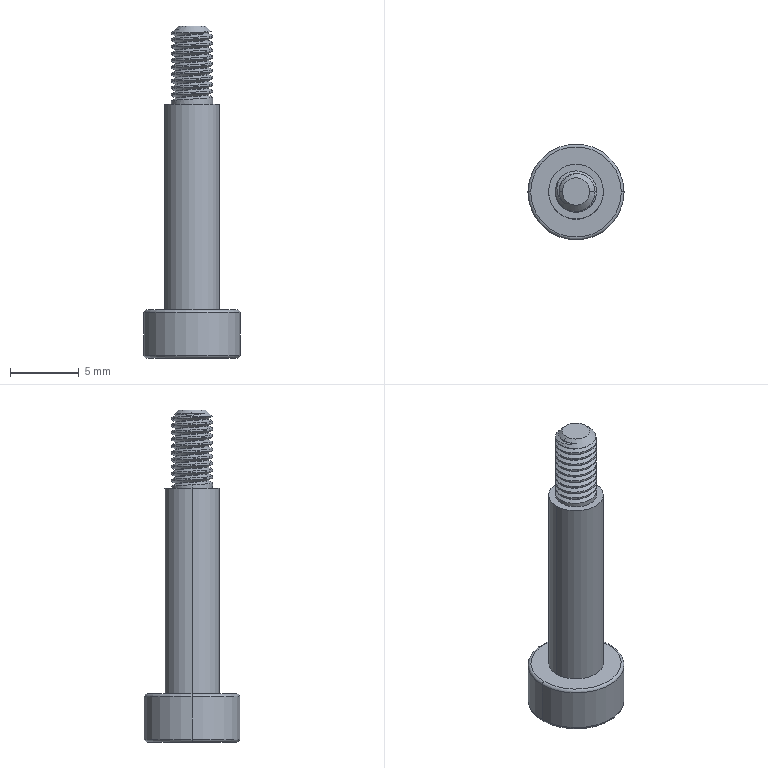Part | SolidWorks | features ICE 3, Chamfer 1, Extrusion 1, Fillet 1, SweepThread 1 | 1 solid | 50 faces | box 7 x 7 x 24.2 mm | volume 319.419 mm3 | cylinder 26 | plane 14 | torus 4 | cone 3 | spline 3 | commonest cylinder face diameters 3 x22 4 x2 7 x2